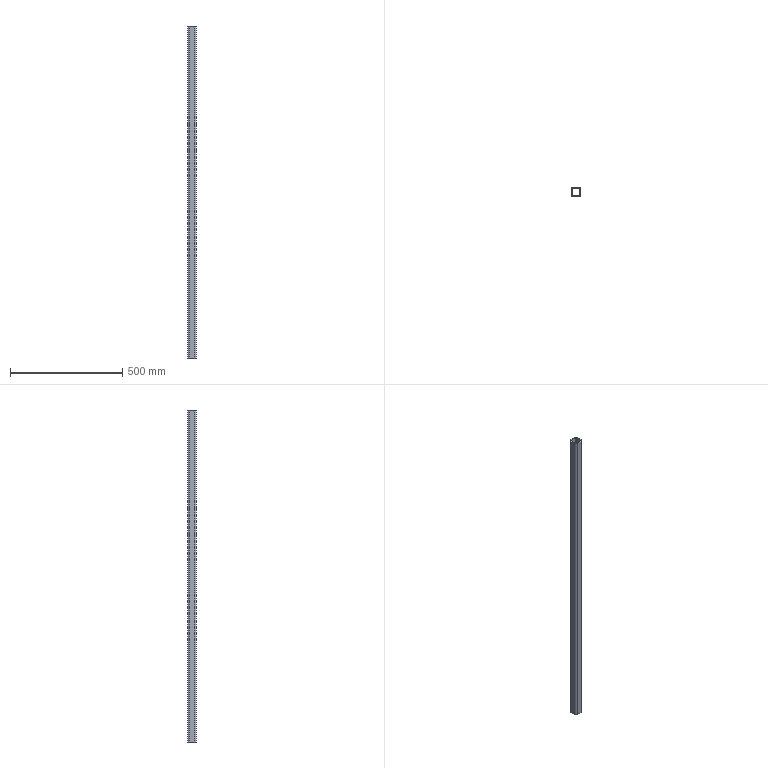Part | STEP file | 40 x 40 x 920 | 1 solid | 18 faces | box 40 x 40 x 1480 mm | volume 791499 mm3 | plane 10 | cylinder 8 | commonest cylinder face diameters 8 x4 16 x4
STEP:
#1=CARTESIAN_POINT('',(0.,32.,-1160.));
#2=VERTEX_POINT('',#1);
#3=CARTESIAN_POINT('',(0.,32.,320.));
#4=VERTEX_POINT('',#3);
#5=CARTESIAN_POINT('',(0.,32.,600.));
#6=DIRECTION('',(0.,0.,1.));
#7=VECTOR('',#6,1000.);
#8=LINE('',#5,#7);
#9=EDGE_CURVE('',#2,#4,#8,.T.);
#10=ORIENTED_EDGE('',*,*,#9,.F.);
#11=CARTESIAN_POINT('',(0.,8.,-1160.));
#12=VERTEX_POINT('',#11);
#13=CARTESIAN_POINT('',(0.,8.,-1160.));
#14=DIRECTION('',(0.,-1.,0.));
#15=VECTOR('',#14,1000.);
#16=LINE('',#13,#15);
#17=EDGE_CURVE('',#2,#12,#16,.T.);
#18=ORIENTED_EDGE('',*,*,#17,.T.);
#19=CARTESIAN_POINT('',(0.,8.,320.));
#20=VERTEX_POINT('',#19);
#21=CARTESIAN_POINT('',(0.,8.,600.));
#22=DIRECTION('',(0.,0.,-1.));
#23=VECTOR('',#22,1000.);
#24=LINE('',#21,#23);
#25=EDGE_CURVE('',#20,#12,#24,.T.);
#26=ORIENTED_EDGE('',*,*,#25,.F.);
#27=CARTESIAN_POINT('',(0.,8.,320.));
#28=DIRECTION('',(0.,-1.,0.));
#29=VECTOR('',#28,1000.);
#30=LINE('',#27,#29);
#31=EDGE_CURVE('',#4,#20,#30,.T.);
#32=ORIENTED_EDGE('',*,*,#31,.F.);
#33=EDGE_LOOP('',(#10,#18,#26,#32));
#34=FACE_OUTER_BOUND('',#33,.T.);
#35=CARTESIAN_POINT('',(0.,8.,600.));
#36=DIRECTION('',(1.,0.,0.));
#37=DIRECTION('',(0.,1.,0.));
#38=AXIS2_PLACEMENT_3D('',#35,#36,#37);
#39=PLANE('',#38);
#40=ADVANCED_FACE('',(#34),#39,.F.);
#41=CARTESIAN_POINT('',(8.,0.,320.));
#42=VERTEX_POINT('',#41);
#43=CARTESIAN_POINT('',(8.,8.,320.));
#44=DIRECTION('',(0.,0.,1.));
#45=DIRECTION('',(-1.,0.,0.));
#46=AXIS2_PLACEMENT_3D('',#43,#44,#45);
#47=CIRCLE('',#46,8.);
#48=EDGE_CURVE('',#20,#42,#47,.T.);
#49=ORIENTED_EDGE('',*,*,#48,.T.);
#50=CARTESIAN_POINT('',(32.,0.,320.));
#51=VERTEX_POINT('',#50);
#52=CARTESIAN_POINT('',(32.,0.,320.));
#53=DIRECTION('',(1.,0.,0.));
#54=VECTOR('',#53,1000.);
#55=LINE('',#52,#54);
#56=EDGE_CURVE('',#42,#51,#55,.T.);
#57=ORIENTED_EDGE('',*,*,#56,.T.);
#58=CARTESIAN_POINT('',(40.,8.,320.));
#59=VERTEX_POINT('',#58);
#60=CARTESIAN_POINT('',(32.,8.,320.));
#61=DIRECTION('',(0.,0.,1.));
#62=DIRECTION('',(-1.,0.,0.));
#63=AXIS2_PLACEMENT_3D('',#60,#61,#62);
#64=CIRCLE('',#63,8.);
#65=EDGE_CURVE('',#51,#59,#64,.T.);
#66=ORIENTED_EDGE('',*,*,#65,.T.);
#67=CARTESIAN_POINT('',(40.,32.,320.));
#68=VERTEX_POINT('',#67);
#69=CARTESIAN_POINT('',(40.,8.,320.));
#70=DIRECTION('',(0.,1.,0.));
#71=VECTOR('',#70,1000.);
#72=LINE('',#69,#71);
#73=EDGE_CURVE('',#59,#68,#72,.T.);
#74=ORIENTED_EDGE('',*,*,#73,.T.);
#75=CARTESIAN_POINT('',(32.,40.,320.));
#76=VERTEX_POINT('',#75);
#77=CARTESIAN_POINT('',(32.,32.,320.));
#78=DIRECTION('',(0.,0.,1.));
#79=DIRECTION('',(-1.,0.,0.));
#80=AXIS2_PLACEMENT_3D('',#77,#78,#79);
#81=CIRCLE('',#80,8.);
#82=EDGE_CURVE('',#68,#76,#81,.T.);
#83=ORIENTED_EDGE('',*,*,#82,.T.);
#84=CARTESIAN_POINT('',(8.,40.,320.));
#85=VERTEX_POINT('',#84);
#86=CARTESIAN_POINT('',(32.,40.,320.));
#87=DIRECTION('',(-1.,0.,0.));
#88=VECTOR('',#87,1000.);
#89=LINE('',#86,#88);
#90=EDGE_CURVE('',#76,#85,#89,.T.);
#91=ORIENTED_EDGE('',*,*,#90,.T.);
#92=CARTESIAN_POINT('',(8.,32.,320.));
#93=DIRECTION('',(0.,0.,1.));
#94=DIRECTION('',(-1.,0.,0.));
#95=AXIS2_PLACEMENT_3D('',#92,#93,#94);
#96=CIRCLE('',#95,8.);
#97=EDGE_CURVE('',#85,#4,#96,.T.);
#98=ORIENTED_EDGE('',*,*,#97,.T.);
#99=ORIENTED_EDGE('',*,*,#31,.T.);
#100=EDGE_LOOP('',(#49,#57,#66,#74,#83,#91,#98,#99));
#101=FACE_OUTER_BOUND('',#100,.T.);
#102=CARTESIAN_POINT('',(4.,32.,320.));
#103=VERTEX_POINT('',#102);
#104=CARTESIAN_POINT('',(8.,36.,320.));
#105=VERTEX_POINT('',#104);
#106=CARTESIAN_POINT('',(8.,32.,320.));
#107=DIRECTION('',(0.,0.,-1.));
#108=DIRECTION('',(-1.,0.,0.));
#109=AXIS2_PLACEMENT_3D('',#106,#107,#108);
#110=CIRCLE('',#109,4.);
#111=EDGE_CURVE('',#103,#105,#110,.T.);
#112=ORIENTED_EDGE('',*,*,#111,.T.);
#113=CARTESIAN_POINT('',(32.,36.,320.));
#114=VERTEX_POINT('',#113);
#115=CARTESIAN_POINT('',(32.,36.,320.));
#116=DIRECTION('',(1.,0.,0.));
#117=VECTOR('',#116,1000.);
#118=LINE('',#115,#117);
#119=EDGE_CURVE('',#105,#114,#118,.T.);
#120=ORIENTED_EDGE('',*,*,#119,.T.);
#121=CARTESIAN_POINT('',(36.,32.,320.));
#122=VERTEX_POINT('',#121);
#123=CARTESIAN_POINT('',(32.,32.,320.));
#124=DIRECTION('',(0.,0.,-1.));
#125=DIRECTION('',(-1.,0.,0.));
#126=AXIS2_PLACEMENT_3D('',#123,#124,#125);
#127=CIRCLE('',#126,4.);
#128=EDGE_CURVE('',#114,#122,#127,.T.);
#129=ORIENTED_EDGE('',*,*,#128,.T.);
#130=CARTESIAN_POINT('',(36.,8.,320.));
#131=VERTEX_POINT('',#130);
#132=CARTESIAN_POINT('',(36.,8.,320.));
#133=DIRECTION('',(0.,-1.,0.));
#134=VECTOR('',#133,1000.);
#135=LINE('',#132,#134);
#136=EDGE_CURVE('',#122,#131,#135,.T.);
#137=ORIENTED_EDGE('',*,*,#136,.T.);
#138=CARTESIAN_POINT('',(32.,4.,320.));
#139=VERTEX_POINT('',#138);
#140=CARTESIAN_POINT('',(32.,8.,320.));
#141=DIRECTION('',(0.,0.,-1.));
#142=DIRECTION('',(-1.,0.,0.));
#143=AXIS2_PLACEMENT_3D('',#140,#141,#142);
#144=CIRCLE('',#143,4.);
#145=EDGE_CURVE('',#131,#139,#144,.T.);
#146=ORIENTED_EDGE('',*,*,#145,.T.);
#147=CARTESIAN_POINT('',(8.,4.,320.));
#148=VERTEX_POINT('',#147);
#149=CARTESIAN_POINT('',(32.,4.,320.));
#150=DIRECTION('',(-1.,0.,0.));
#151=VECTOR('',#150,1000.);
#152=LINE('',#149,#151);
#153=EDGE_CURVE('',#139,#148,#152,.T.);
#154=ORIENTED_EDGE('',*,*,#153,.T.);
#155=CARTESIAN_POINT('',(4.,8.,320.));
#156=VERTEX_POINT('',#155);
#157=CARTESIAN_POINT('',(8.,8.,320.));
#158=DIRECTION('',(0.,0.,-1.));
#159=DIRECTION('',(-1.,0.,0.));
#160=AXIS2_PLACEMENT_3D('',#157,#158,#159);
#161=CIRCLE('',#160,4.);
#162=EDGE_CURVE('',#148,#156,#161,.T.);
#163=ORIENTED_EDGE('',*,*,#162,.T.);
#164=CARTESIAN_POINT('',(4.,8.,320.));
#165=DIRECTION('',(0.,1.,0.));
#166=VECTOR('',#165,1000.);
#167=LINE('',#164,#166);
#168=EDGE_CURVE('',#156,#103,#167,.T.);
#169=ORIENTED_EDGE('',*,*,#168,.T.);
#170=EDGE_LOOP('',(#112,#120,#129,#137,#146,#154,#163,#169));
#171=FACE_BOUND('',#170,.T.);
#172=CARTESIAN_POINT('',(32.,8.,320.));
#173=DIRECTION('',(0.,0.,1.));
#174=DIRECTION('',(1.,0.,0.));
#175=AXIS2_PLACEMENT_3D('',#172,#173,#174);
#176=PLANE('',#175);
#177=ADVANCED_FACE('',(#101,#171),#176,.T.);
#178=CARTESIAN_POINT('',(8.,40.,-1160.));
#179=VERTEX_POINT('',#178);
#180=CARTESIAN_POINT('',(8.,40.,600.));
#181=DIRECTION('',(0.,0.,-1.));
#182=VECTOR('',#181,1000.);
#183=LINE('',#180,#182);
#184=EDGE_CURVE('',#85,#179,#183,.T.);
#185=ORIENTED_EDGE('',*,*,#184,.T.);
#186=CARTESIAN_POINT('',(8.,32.,-1160.));
#187=DIRECTION('',(0.,0.,1.));
#188=DIRECTION('',(1.,0.,0.));
#189=AXIS2_PLACEMENT_3D('',#186,#187,#188);
#190=CIRCLE('',#189,8.);
#191=EDGE_CURVE('',#179,#2,#190,.T.);
#192=ORIENTED_EDGE('',*,*,#191,.T.);
#193=ORIENTED_EDGE('',*,*,#9,.T.);
#194=ORIENTED_EDGE('',*,*,#97,.F.);
#195=EDGE_LOOP('',(#185,#192,#193,#194));
#196=FACE_OUTER_BOUND('',#195,.T.);
#197=CARTESIAN_POINT('',(8.,32.,600.));
#198=DIRECTION('',(0.,0.,-1.));
#199=DIRECTION('',(-1.,0.,0.));
#200=AXIS2_PLACEMENT_3D('',#197,#198,#199);
#201=CYLINDRICAL_SURFACE('',#200,8.);
#202=ADVANCED_FACE('',(#196),#201,.T.);
#203=ORIENTED_EDGE('',*,*,#25,.T.);
#204=CARTESIAN_POINT('',(8.,0.,-1160.));
#205=VERTEX_POINT('',#204);
#206=CARTESIAN_POINT('',(8.,8.,-1160.));
#207=DIRECTION('',(0.,0.,1.));
#208=DIRECTION('',(1.,0.,0.));
#209=AXIS2_PLACEMENT_3D('',#206,#207,#208);
#210=CIRCLE('',#209,8.);
#211=EDGE_CURVE('',#12,#205,#210,.T.);
#212=ORIENTED_EDGE('',*,*,#211,.T.);
#213=CARTESIAN_POINT('',(8.,0.,600.));
#214=DIRECTION('',(0.,0.,1.));
#215=VECTOR('',#214,1000.);
#216=LINE('',#213,#215);
#217=EDGE_CURVE('',#205,#42,#216,.T.);
#218=ORIENTED_EDGE('',*,*,#217,.T.);
#219=ORIENTED_EDGE('',*,*,#48,.F.);
#220=EDGE_LOOP('',(#203,#212,#218,#219));
#221=FACE_OUTER_BOUND('',#220,.T.);
#222=CARTESIAN_POINT('',(8.,8.,600.));
#223=DIRECTION('',(0.,0.,-1.));
#224=DIRECTION('',(-1.,0.,0.));
#225=AXIS2_PLACEMENT_3D('',#222,#223,#224);
#226=CYLINDRICAL_SURFACE('',#225,8.);
#227=ADVANCED_FACE('',(#221),#226,.T.);
#228=ORIENTED_EDGE('',*,*,#217,.F.);
#229=CARTESIAN_POINT('',(32.,0.,-1160.));
#230=VERTEX_POINT('',#229);
#231=CARTESIAN_POINT('',(32.,0.,-1160.));
#232=DIRECTION('',(1.,0.,0.));
#233=VECTOR('',#232,1000.);
#234=LINE('',#231,#233);
#235=EDGE_CURVE('',#205,#230,#234,.T.);
#236=ORIENTED_EDGE('',*,*,#235,.T.);
#237=CARTESIAN_POINT('',(32.,0.,600.));
#238=DIRECTION('',(0.,0.,-1.));
#239=VECTOR('',#238,1000.);
#240=LINE('',#237,#239);
#241=EDGE_CURVE('',#51,#230,#240,.T.);
#242=ORIENTED_EDGE('',*,*,#241,.F.);
#243=ORIENTED_EDGE('',*,*,#56,.F.);
#244=EDGE_LOOP('',(#228,#236,#242,#243));
#245=FACE_OUTER_BOUND('',#244,.T.);
#246=CARTESIAN_POINT('',(8.,0.,600.));
#247=DIRECTION('',(0.,1.,0.));
#248=DIRECTION('',(-1.,0.,0.));
#249=AXIS2_PLACEMENT_3D('',#246,#247,#248);
#250=PLANE('',#249);
#251=ADVANCED_FACE('',(#245),#250,.F.);
#252=CARTESIAN_POINT('',(32.,40.,-1160.));
#253=VERTEX_POINT('',#252);
#254=CARTESIAN_POINT('',(32.,40.,600.));
#255=DIRECTION('',(0.,0.,1.));
#256=VECTOR('',#255,1000.);
#257=LINE('',#254,#256);
#258=EDGE_CURVE('',#253,#76,#257,.T.);
#259=ORIENTED_EDGE('',*,*,#258,.F.);
#260=CARTESIAN_POINT('',(8.,40.,-1160.));
#261=DIRECTION('',(-1.,0.,0.));
#262=VECTOR('',#261,1000.);
#263=LINE('',#260,#262);
#264=EDGE_CURVE('',#253,#179,#263,.T.);
#265=ORIENTED_EDGE('',*,*,#264,.T.);
#266=ORIENTED_EDGE('',*,*,#184,.F.);
#267=ORIENTED_EDGE('',*,*,#90,.F.);
#268=EDGE_LOOP('',(#259,#265,#266,#267));
#269=FACE_OUTER_BOUND('',#268,.T.);
#270=CARTESIAN_POINT('',(32.,40.,600.));
#271=DIRECTION('',(0.,-1.,0.));
#272=DIRECTION('',(1.,0.,0.));
#273=AXIS2_PLACEMENT_3D('',#270,#271,#272);
#274=PLANE('',#273);
#275=ADVANCED_FACE('',(#269),#274,.F.);
#276=CARTESIAN_POINT('',(40.,32.,-1160.));
#277=VERTEX_POINT('',#276);
#278=CARTESIAN_POINT('',(40.,32.,600.));
#279=DIRECTION('',(0.,0.,-1.));
#280=VECTOR('',#279,1000.);
#281=LINE('',#278,#280);
#282=EDGE_CURVE('',#68,#277,#281,.T.);
#283=ORIENTED_EDGE('',*,*,#282,.T.);
#284=CARTESIAN_POINT('',(32.,32.,-1160.));
#285=DIRECTION('',(0.,0.,1.));
#286=DIRECTION('',(1.,0.,0.));
#287=AXIS2_PLACEMENT_3D('',#284,#285,#286);
#288=CIRCLE('',#287,8.);
#289=EDGE_CURVE('',#277,#253,#288,.T.);
#290=ORIENTED_EDGE('',*,*,#289,.T.);
#291=ORIENTED_EDGE('',*,*,#258,.T.);
#292=ORIENTED_EDGE('',*,*,#82,.F.);
#293=EDGE_LOOP('',(#283,#290,#291,#292));
#294=FACE_OUTER_BOUND('',#293,.T.);
#295=CARTESIAN_POINT('',(32.,32.,600.));
#296=DIRECTION('',(0.,0.,-1.));
#297=DIRECTION('',(-1.,0.,0.));
#298=AXIS2_PLACEMENT_3D('',#295,#296,#297);
#299=CYLINDRICAL_SURFACE('',#298,8.);
#300=ADVANCED_FACE('',(#294),#299,.T.);
#301=CARTESIAN_POINT('',(40.,8.,-1160.));
#302=VERTEX_POINT('',#301);
#303=CARTESIAN_POINT('',(40.,8.,600.));
#304=DIRECTION('',(0.,0.,1.));
#305=VECTOR('',#304,1000.);
#306=LINE('',#303,#305);
#307=EDGE_CURVE('',#302,#59,#306,.T.);
#308=ORIENTED_EDGE('',*,*,#307,.F.);
#309=CARTESIAN_POINT('',(40.,32.,-1160.));
#310=DIRECTION('',(0.,1.,0.));
#311=VECTOR('',#310,1000.);
#312=LINE('',#309,#311);
#313=EDGE_CURVE('',#302,#277,#312,.T.);
#314=ORIENTED_EDGE('',*,*,#313,.T.);
#315=ORIENTED_EDGE('',*,*,#282,.F.);
#316=ORIENTED_EDGE('',*,*,#73,.F.);
#317=EDGE_LOOP('',(#308,#314,#315,#316));
#318=FACE_OUTER_BOUND('',#317,.T.);
#319=CARTESIAN_POINT('',(40.,32.,600.));
#320=DIRECTION('',(-1.,0.,0.));
#321=DIRECTION('',(0.,-1.,0.));
#322=AXIS2_PLACEMENT_3D('',#319,#320,#321);
#323=PLANE('',#322);
#324=ADVANCED_FACE('',(#318),#323,.F.);
#325=ORIENTED_EDGE('',*,*,#241,.T.);
#326=CARTESIAN_POINT('',(32.,8.,-1160.));
#327=DIRECTION('',(0.,0.,1.));
#328=DIRECTION('',(1.,0.,0.));
#329=AXIS2_PLACEMENT_3D('',#326,#327,#328);
#330=CIRCLE('',#329,8.);
#331=EDGE_CURVE('',#230,#302,#330,.T.);
#332=ORIENTED_EDGE('',*,*,#331,.T.);
#333=ORIENTED_EDGE('',*,*,#307,.T.);
#334=ORIENTED_EDGE('',*,*,#65,.F.);
#335=EDGE_LOOP('',(#325,#332,#333,#334));
#336=FACE_OUTER_BOUND('',#335,.T.);
#337=CARTESIAN_POINT('',(32.,8.,600.));
#338=DIRECTION('',(0.,0.,-1.));
#339=DIRECTION('',(-1.,0.,0.));
#340=AXIS2_PLACEMENT_3D('',#337,#338,#339);
#341=CYLINDRICAL_SURFACE('',#340,8.);
#342=ADVANCED_FACE('',(#336),#341,.T.);
#343=CARTESIAN_POINT('',(8.,36.,-1160.));
#344=VERTEX_POINT('',#343);
#345=CARTESIAN_POINT('',(8.,36.,600.));
#346=DIRECTION('',(0.,0.,-1.));
#347=VECTOR('',#346,1000.);
#348=LINE('',#345,#347);
#349=EDGE_CURVE('',#105,#344,#348,.T.);
#350=ORIENTED_EDGE('',*,*,#349,.T.);
#351=CARTESIAN_POINT('',(32.,36.,-1160.));
#352=VERTEX_POINT('',#351);
#353=CARTESIAN_POINT('',(8.,36.,-1160.));
#354=DIRECTION('',(-1.,0.,0.));
#355=VECTOR('',#354,1000.);
#356=LINE('',#353,#355);
#357=EDGE_CURVE('',#352,#344,#356,.T.);
#358=ORIENTED_EDGE('',*,*,#357,.F.);
#359=CARTESIAN_POINT('',(32.,36.,600.));
#360=DIRECTION('',(0.,0.,1.));
#361=VECTOR('',#360,1000.);
#362=LINE('',#359,#361);
#363=EDGE_CURVE('',#352,#114,#362,.T.);
#364=ORIENTED_EDGE('',*,*,#363,.T.);
#365=ORIENTED_EDGE('',*,*,#119,.F.);
#366=EDGE_LOOP('',(#350,#358,#364,#365));
#367=FACE_OUTER_BOUND('',#366,.T.);
#368=CARTESIAN_POINT('',(32.,36.,600.));
#369=DIRECTION('',(0.,-1.,0.));
#370=DIRECTION('',(0.,0.,-1.));
#371=AXIS2_PLACEMENT_3D('',#368,#369,#370);
#372=PLANE('',#371);
#373=ADVANCED_FACE('',(#367),#372,.T.);
#374=CARTESIAN_POINT('',(4.,32.,-1160.));
#375=VERTEX_POINT('',#374);
#376=CARTESIAN_POINT('',(4.,32.,600.));
#377=DIRECTION('',(0.,0.,1.));
#378=VECTOR('',#377,1000.);
#379=LINE('',#376,#378);
#380=EDGE_CURVE('',#375,#103,#379,.T.);
#381=ORIENTED_EDGE('',*,*,#380,.F.);
#382=CARTESIAN_POINT('',(8.,32.,-1160.));
#383=DIRECTION('',(0.,0.,1.));
#384=DIRECTION('',(1.,0.,0.));
#385=AXIS2_PLACEMENT_3D('',#382,#383,#384);
#386=CIRCLE('',#385,4.);
#387=EDGE_CURVE('',#344,#375,#386,.T.);
#388=ORIENTED_EDGE('',*,*,#387,.F.);
#389=ORIENTED_EDGE('',*,*,#349,.F.);
#390=ORIENTED_EDGE('',*,*,#111,.F.);
#391=EDGE_LOOP('',(#381,#388,#389,#390));
#392=FACE_OUTER_BOUND('',#391,.T.);
#393=CARTESIAN_POINT('',(8.,32.,600.));
#394=DIRECTION('',(0.,0.,-1.));
#395=DIRECTION('',(-1.,0.,0.));
#396=AXIS2_PLACEMENT_3D('',#393,#394,#395);
#397=CYLINDRICAL_SURFACE('',#396,4.);
#398=ADVANCED_FACE('',(#392),#397,.F.);
#399=CARTESIAN_POINT('',(4.,8.,-1160.));
#400=VERTEX_POINT('',#399);
#401=CARTESIAN_POINT('',(4.,8.,600.));
#402=DIRECTION('',(0.,0.,-1.));
#403=VECTOR('',#402,1000.);
#404=LINE('',#401,#403);
#405=EDGE_CURVE('',#156,#400,#404,.T.);
#406=ORIENTED_EDGE('',*,*,#405,.T.);
#407=CARTESIAN_POINT('',(4.,8.,-1160.));
#408=DIRECTION('',(0.,-1.,0.));
#409=VECTOR('',#408,1000.);
#410=LINE('',#407,#409);
#411=EDGE_CURVE('',#375,#400,#410,.T.);
#412=ORIENTED_EDGE('',*,*,#411,.F.);
#413=ORIENTED_EDGE('',*,*,#380,.T.);
#414=ORIENTED_EDGE('',*,*,#168,.F.);
#415=EDGE_LOOP('',(#406,#412,#413,#414));
#416=FACE_OUTER_BOUND('',#415,.T.);
#417=CARTESIAN_POINT('',(4.,8.,600.));
#418=DIRECTION('',(1.,0.,0.));
#419=DIRECTION('',(0.,1.,0.));
#420=AXIS2_PLACEMENT_3D('',#417,#418,#419);
#421=PLANE('',#420);
#422=ADVANCED_FACE('',(#416),#421,.T.);
#423=CARTESIAN_POINT('',(8.,4.,-1160.));
#424=VERTEX_POINT('',#423);
#425=CARTESIAN_POINT('',(8.,4.,600.));
#426=DIRECTION('',(0.,0.,1.));
#427=VECTOR('',#426,1000.);
#428=LINE('',#425,#427);
#429=EDGE_CURVE('',#424,#148,#428,.T.);
#430=ORIENTED_EDGE('',*,*,#429,.F.);
#431=CARTESIAN_POINT('',(8.,8.,-1160.));
#432=DIRECTION('',(0.,0.,1.));
#433=DIRECTION('',(1.,0.,0.));
#434=AXIS2_PLACEMENT_3D('',#431,#432,#433);
#435=CIRCLE('',#434,4.);
#436=EDGE_CURVE('',#400,#424,#435,.T.);
#437=ORIENTED_EDGE('',*,*,#436,.F.);
#438=ORIENTED_EDGE('',*,*,#405,.F.);
#439=ORIENTED_EDGE('',*,*,#162,.F.);
#440=EDGE_LOOP('',(#430,#437,#438,#439));
#441=FACE_OUTER_BOUND('',#440,.T.);
#442=CARTESIAN_POINT('',(8.,8.,600.));
#443=DIRECTION('',(0.,0.,-1.));
#444=DIRECTION('',(-1.,0.,0.));
#445=AXIS2_PLACEMENT_3D('',#442,#443,#444);
#446=CYLINDRICAL_SURFACE('',#445,4.);
#447=ADVANCED_FACE('',(#441),#446,.F.);
#448=CARTESIAN_POINT('',(32.,4.,-1160.));
#449=VERTEX_POINT('',#448);
#450=CARTESIAN_POINT('',(32.,4.,600.));
#451=DIRECTION('',(0.,0.,-1.));
#452=VECTOR('',#451,1000.);
#453=LINE('',#450,#452);
#454=EDGE_CURVE('',#139,#449,#453,.T.);
#455=ORIENTED_EDGE('',*,*,#454,.T.);
#456=CARTESIAN_POINT('',(32.,4.,-1160.));
#457=DIRECTION('',(1.,0.,0.));
#458=VECTOR('',#457,1000.);
#459=LINE('',#456,#458);
#460=EDGE_CURVE('',#424,#449,#459,.T.);
#461=ORIENTED_EDGE('',*,*,#460,.F.);
#462=ORIENTED_EDGE('',*,*,#429,.T.);
#463=ORIENTED_EDGE('',*,*,#153,.F.);
#464=EDGE_LOOP('',(#455,#461,#462,#463));
#465=FACE_OUTER_BOUND('',#464,.T.);
#466=CARTESIAN_POINT('',(8.,4.,600.));
#467=DIRECTION('',(0.,1.,0.));
#468=DIRECTION('',(-1.,0.,0.));
#469=AXIS2_PLACEMENT_3D('',#466,#467,#468);
#470=PLANE('',#469);
#471=ADVANCED_FACE('',(#465),#470,.T.);
#472=CARTESIAN_POINT('',(36.,8.,-1160.));
#473=VERTEX_POINT('',#472);
#474=CARTESIAN_POINT('',(36.,8.,600.));
#475=DIRECTION('',(0.,0.,1.));
#476=VECTOR('',#475,1000.);
#477=LINE('',#474,#476);
#478=EDGE_CURVE('',#473,#131,#477,.T.);
#479=ORIENTED_EDGE('',*,*,#478,.F.);
#480=CARTESIAN_POINT('',(32.,8.,-1160.));
#481=DIRECTION('',(0.,0.,1.));
#482=DIRECTION('',(1.,0.,0.));
#483=AXIS2_PLACEMENT_3D('',#480,#481,#482);
#484=CIRCLE('',#483,4.);
#485=EDGE_CURVE('',#449,#473,#484,.T.);
#486=ORIENTED_EDGE('',*,*,#485,.F.);
#487=ORIENTED_EDGE('',*,*,#454,.F.);
#488=ORIENTED_EDGE('',*,*,#145,.F.);
#489=EDGE_LOOP('',(#479,#486,#487,#488));
#490=FACE_OUTER_BOUND('',#489,.T.);
#491=CARTESIAN_POINT('',(32.,8.,600.));
#492=DIRECTION('',(0.,0.,-1.));
#493=DIRECTION('',(-1.,0.,0.));
#494=AXIS2_PLACEMENT_3D('',#491,#492,#493);
#495=CYLINDRICAL_SURFACE('',#494,4.);
#496=ADVANCED_FACE('',(#490),#495,.F.);
#497=CARTESIAN_POINT('',(36.,32.,-1160.));
#498=VERTEX_POINT('',#497);
#499=CARTESIAN_POINT('',(36.,32.,600.));
#500=DIRECTION('',(0.,0.,-1.));
#501=VECTOR('',#500,1000.);
#502=LINE('',#499,#501);
#503=EDGE_CURVE('',#122,#498,#502,.T.);
#504=ORIENTED_EDGE('',*,*,#503,.T.);
#505=CARTESIAN_POINT('',(36.,32.,-1160.));
#506=DIRECTION('',(0.,1.,0.));
#507=VECTOR('',#506,1000.);
#508=LINE('',#505,#507);
#509=EDGE_CURVE('',#473,#498,#508,.T.);
#510=ORIENTED_EDGE('',*,*,#509,.F.);
#511=ORIENTED_EDGE('',*,*,#478,.T.);
#512=ORIENTED_EDGE('',*,*,#136,.F.);
#513=EDGE_LOOP('',(#504,#510,#511,#512));
#514=FACE_OUTER_BOUND('',#513,.T.);
#515=CARTESIAN_POINT('',(36.,32.,600.));
#516=DIRECTION('',(-1.,0.,0.));
#517=DIRECTION('',(0.,0.,1.));
#518=AXIS2_PLACEMENT_3D('',#515,#516,#517);
#519=PLANE('',#518);
#520=ADVANCED_FACE('',(#514),#519,.T.);
#521=ORIENTED_EDGE('',*,*,#363,.F.);
#522=CARTESIAN_POINT('',(32.,32.,-1160.));
#523=DIRECTION('',(0.,0.,1.));
#524=DIRECTION('',(1.,0.,0.));
#525=AXIS2_PLACEMENT_3D('',#522,#523,#524);
#526=CIRCLE('',#525,4.);
#527=EDGE_CURVE('',#498,#352,#526,.T.);
#528=ORIENTED_EDGE('',*,*,#527,.F.);
#529=ORIENTED_EDGE('',*,*,#503,.F.);
#530=ORIENTED_EDGE('',*,*,#128,.F.);
#531=EDGE_LOOP('',(#521,#528,#529,#530));
#532=FACE_OUTER_BOUND('',#531,.T.);
#533=CARTESIAN_POINT('',(32.,32.,600.));
#534=DIRECTION('',(0.,0.,-1.));
#535=DIRECTION('',(-1.,0.,0.));
#536=AXIS2_PLACEMENT_3D('',#533,#534,#535);
#537=CYLINDRICAL_SURFACE('',#536,4.);
#538=ADVANCED_FACE('',(#532),#537,.F.);
#539=ORIENTED_EDGE('',*,*,#387,.T.);
#540=ORIENTED_EDGE('',*,*,#411,.T.);
#541=ORIENTED_EDGE('',*,*,#436,.T.);
#542=ORIENTED_EDGE('',*,*,#460,.T.);
#543=ORIENTED_EDGE('',*,*,#485,.T.);
#544=ORIENTED_EDGE('',*,*,#509,.T.);
#545=ORIENTED_EDGE('',*,*,#527,.T.);
#546=ORIENTED_EDGE('',*,*,#357,.T.);
#547=EDGE_LOOP('',(#539,#540,#541,#542,#543,#544,#545,#546));
#548=FACE_BOUND('',#547,.T.);
#549=ORIENTED_EDGE('',*,*,#235,.F.);
#550=ORIENTED_EDGE('',*,*,#211,.F.);
#551=ORIENTED_EDGE('',*,*,#17,.F.);
#552=ORIENTED_EDGE('',*,*,#191,.F.);
#553=ORIENTED_EDGE('',*,*,#264,.F.);
#554=ORIENTED_EDGE('',*,*,#289,.F.);
#555=ORIENTED_EDGE('',*,*,#313,.F.);
#556=ORIENTED_EDGE('',*,*,#331,.F.);
#557=EDGE_LOOP('',(#549,#550,#551,#552,#553,#554,#555,#556));
#558=FACE_OUTER_BOUND('',#557,.T.);
#559=CARTESIAN_POINT('',(-1450.,-56.,-1160.));
#560=DIRECTION('',(0.,0.,1.));
#561=DIRECTION('',(0.,1.,0.));
#562=AXIS2_PLACEMENT_3D('',#559,#560,#561);
#563=PLANE('',#562);
#564=ADVANCED_FACE('',(#548,#558),#563,.F.);
#565=CLOSED_SHELL('',(#40,#177,#202,#227,#251,#275,#300,#324,#342,#373,#398,#422,#447,#471,#496,#520,#538,#564));
#566=MANIFOLD_SOLID_BREP('',#565);
#567=CARTESIAN_POINT('',(0.,0.,0.));
#568=DIRECTION('',(0.,0.,1.));
#569=DIRECTION('',(1.,0.,0.));
#570=AXIS2_PLACEMENT_3D('',#567,#568,#569);
#571=(LENGTH_UNIT()NAMED_UNIT(*)SI_UNIT(.MILLI.,.METRE.));
#572=UNCERTAINTY_MEASURE_WITH_UNIT(LENGTH_MEASURE(0.00001),#571,'','');
#573=(NAMED_UNIT(*)PLANE_ANGLE_UNIT()SI_UNIT($,.RADIAN.));
#574=(NAMED_UNIT(*)SI_UNIT($,.STERADIAN.)SOLID_ANGLE_UNIT());
#575=(GEOMETRIC_REPRESENTATION_CONTEXT(3)GLOBAL_UNCERTAINTY_ASSIGNED_CONTEXT((#572))GLOBAL_UNIT_ASSIGNED_CONTEXT((#571,#573,#574))REPRESENTATION_CONTEXT('',''));
#576=ADVANCED_BREP_SHAPE_REPRESENTATION('',(#566,#570),#575);